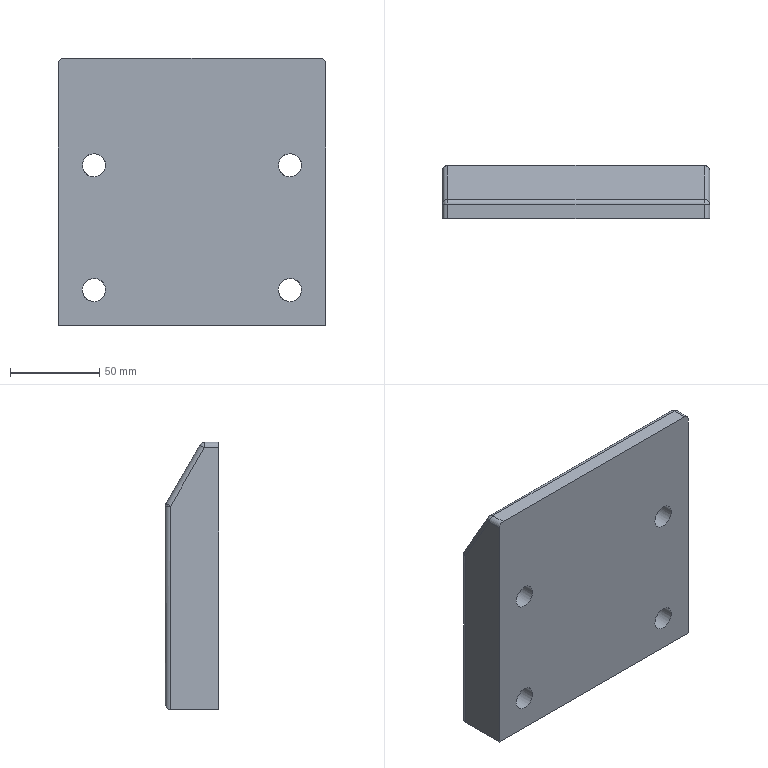Part | NX | features solid 2 | 1 solid | 36 faces | box 150 x 30 x 150 mm | volume 593626 mm3 | cylinder 17 | plane 11 | torus 4 | sphere 4 | commonest cylinder face diameters 6 x9 13 x4 20 x4
STEP:
#1=CARTESIAN_POINT('',(246.5,-620.,-266.5));
#2=VERTEX_POINT('',#1);
#3=CARTESIAN_POINT('',(246.5,-620.,-260.));
#4=DIRECTION('',(0.,1.,0.));
#5=DIRECTION('',(0.,0.,-1.));
#6=AXIS2_PLACEMENT_3D('',#3,#4,#5);
#7=CIRCLE('',#6,6.5);
#8=EDGE_CURVE('',#2,#2,#7,.F.);
#9=ORIENTED_EDGE('',*,*,#8,.F.);
#10=EDGE_LOOP('',(#9));
#11=FACE_BOUND('',#10,.T.);
#12=CARTESIAN_POINT('',(136.5,-620.,-266.5));
#13=VERTEX_POINT('',#12);
#14=CARTESIAN_POINT('',(136.5,-620.,-260.));
#15=DIRECTION('',(0.,1.,0.));
#16=DIRECTION('',(0.,0.,-1.));
#17=AXIS2_PLACEMENT_3D('',#14,#15,#16);
#18=CIRCLE('',#17,6.5);
#19=EDGE_CURVE('',#13,#13,#18,.F.);
#20=ORIENTED_EDGE('',*,*,#19,.F.);
#21=EDGE_LOOP('',(#20));
#22=FACE_BOUND('',#21,.T.);
#23=CARTESIAN_POINT('',(116.5,-620.,-133.));
#24=VERTEX_POINT('',#23);
#25=CARTESIAN_POINT('',(116.5,-620.,-280.));
#26=VERTEX_POINT('',#25);
#27=CARTESIAN_POINT('',(116.5,-620.,-40.));
#28=DIRECTION('',(0.,0.,-1.));
#29=VECTOR('',#28,1000.);
#30=LINE('',#27,#29);
#31=EDGE_CURVE('',#24,#26,#30,.T.);
#32=ORIENTED_EDGE('',*,*,#31,.T.);
#33=CARTESIAN_POINT('',(266.5,-620.,-280.));
#34=VERTEX_POINT('',#33);
#35=CARTESIAN_POINT('',(229.,-620.,-280.));
#36=DIRECTION('',(1.,0.,0.));
#37=VECTOR('',#36,1000.);
#38=LINE('',#35,#37);
#39=EDGE_CURVE('',#26,#34,#38,.T.);
#40=ORIENTED_EDGE('',*,*,#39,.T.);
#41=CARTESIAN_POINT('',(266.5,-620.,-133.));
#42=VERTEX_POINT('',#41);
#43=CARTESIAN_POINT('',(266.5,-620.,-40.));
#44=DIRECTION('',(0.,0.,-1.));
#45=VECTOR('',#44,1000.);
#46=LINE('',#43,#45);
#47=EDGE_CURVE('',#42,#34,#46,.T.);
#48=ORIENTED_EDGE('',*,*,#47,.F.);
#49=CARTESIAN_POINT('',(263.5,-620.,-130.));
#50=VERTEX_POINT('',#49);
#51=CARTESIAN_POINT('',(263.5,-620.,-133.));
#52=DIRECTION('',(0.,1.,0.));
#53=DIRECTION('',(0.,0.,-1.));
#54=AXIS2_PLACEMENT_3D('',#51,#52,#53);
#55=CIRCLE('',#54,3.);
#56=EDGE_CURVE('',#42,#50,#55,.F.);
#57=ORIENTED_EDGE('',*,*,#56,.T.);
#58=CARTESIAN_POINT('',(119.5,-620.,-130.));
#59=VERTEX_POINT('',#58);
#60=CARTESIAN_POINT('',(229.,-620.,-130.));
#61=DIRECTION('',(-1.,0.,0.));
#62=VECTOR('',#61,1000.);
#63=LINE('',#60,#62);
#64=EDGE_CURVE('',#50,#59,#63,.T.);
#65=ORIENTED_EDGE('',*,*,#64,.T.);
#66=CARTESIAN_POINT('',(119.5,-620.,-133.));
#67=DIRECTION('',(0.,1.,0.));
#68=DIRECTION('',(0.,0.,-1.));
#69=AXIS2_PLACEMENT_3D('',#66,#67,#68);
#70=CIRCLE('',#69,3.);
#71=EDGE_CURVE('',#59,#24,#70,.F.);
#72=ORIENTED_EDGE('',*,*,#71,.T.);
#73=EDGE_LOOP('',(#32,#40,#48,#57,#65,#72));
#74=FACE_BOUND('',#73,.T.);
#75=CARTESIAN_POINT('',(246.5,-620.,-196.5));
#76=VERTEX_POINT('',#75);
#77=CARTESIAN_POINT('',(246.5,-620.,-190.));
#78=DIRECTION('',(0.,1.,0.));
#79=DIRECTION('',(0.,0.,-1.));
#80=AXIS2_PLACEMENT_3D('',#77,#78,#79);
#81=CIRCLE('',#80,6.5);
#82=EDGE_CURVE('',#76,#76,#81,.F.);
#83=ORIENTED_EDGE('',*,*,#82,.F.);
#84=EDGE_LOOP('',(#83));
#85=FACE_BOUND('',#84,.T.);
#86=CARTESIAN_POINT('',(136.5,-620.,-196.5));
#87=VERTEX_POINT('',#86);
#88=CARTESIAN_POINT('',(136.5,-620.,-190.));
#89=DIRECTION('',(0.,1.,0.));
#90=DIRECTION('',(0.,0.,-1.));
#91=AXIS2_PLACEMENT_3D('',#88,#89,#90);
#92=CIRCLE('',#91,6.5);
#93=EDGE_CURVE('',#87,#87,#92,.F.);
#94=ORIENTED_EDGE('',*,*,#93,.F.);
#95=EDGE_LOOP('',(#94));
#96=FACE_BOUND('',#95,.T.);
#97=CARTESIAN_POINT('',(-795.,-620.,-162.208));
#98=DIRECTION('',(0.,-1.,0.));
#99=DIRECTION('',(0.,0.,-1.));
#100=AXIS2_PLACEMENT_3D('',#97,#98,#99);
#101=PLANE('',#100);
#102=ADVANCED_FACE('',(#11,#22,#74,#85,#96),#101,.T.);
#103=CARTESIAN_POINT('',(119.5,-590.,-165.804));
#104=VERTEX_POINT('',#103);
#105=CARTESIAN_POINT('',(119.5,-590.,-277.));
#106=VERTEX_POINT('',#105);
#107=CARTESIAN_POINT('',(119.5,-590.,-170.));
#108=DIRECTION('',(0.,0.,1.));
#109=VECTOR('',#108,1000.);
#110=LINE('',#107,#109);
#111=EDGE_CURVE('',#104,#106,#110,.F.);
#112=ORIENTED_EDGE('',*,*,#111,.T.);
#113=CARTESIAN_POINT('',(116.5,-593.,-280.));
#114=VERTEX_POINT('',#113);
#115=CARTESIAN_POINT('',(119.5,-593.,-277.));
#116=DIRECTION('',(0.7071,0.,-0.7071));
#117=DIRECTION('',(-0.7071,0.,-0.7071));
#118=AXIS2_PLACEMENT_3D('',#115,#116,#117);
#119=ELLIPSE('',#118,4.243,3.);
#120=EDGE_CURVE('',#114,#106,#119,.T.);
#121=ORIENTED_EDGE('',*,*,#120,.F.);
#122=CARTESIAN_POINT('',(116.5,-593.,-165.804));
#123=VERTEX_POINT('',#122);
#124=CARTESIAN_POINT('',(116.5,-593.,-40.));
#125=DIRECTION('',(0.,0.,1.));
#126=VECTOR('',#125,1000.);
#127=LINE('',#124,#126);
#128=EDGE_CURVE('',#114,#123,#127,.T.);
#129=ORIENTED_EDGE('',*,*,#128,.T.);
#130=CARTESIAN_POINT('',(119.5,-593.,-165.804));
#131=DIRECTION('',(0.,0.,-1.));
#132=DIRECTION('',(-1.,0.,0.));
#133=AXIS2_PLACEMENT_3D('',#130,#131,#132);
#134=CIRCLE('',#133,3.);
#135=EDGE_CURVE('',#104,#123,#134,.F.);
#136=ORIENTED_EDGE('',*,*,#135,.F.);
#137=EDGE_LOOP('',(#112,#121,#129,#136));
#138=FACE_BOUND('',#137,.T.);
#139=CARTESIAN_POINT('',(119.5,-593.,-40.));
#140=DIRECTION('',(0.,0.,1.));
#141=DIRECTION('',(-1.,0.,0.));
#142=AXIS2_PLACEMENT_3D('',#139,#140,#141);
#143=CYLINDRICAL_SURFACE('',#142,3.);
#144=ADVANCED_FACE('',(#138),#143,.T.);
#145=CARTESIAN_POINT('',(266.5,-593.,-165.804));
#146=VERTEX_POINT('',#145);
#147=CARTESIAN_POINT('',(266.5,-593.,-280.));
#148=VERTEX_POINT('',#147);
#149=CARTESIAN_POINT('',(266.5,-593.,-170.));
#150=DIRECTION('',(0.,0.,1.));
#151=VECTOR('',#150,1000.);
#152=LINE('',#149,#151);
#153=EDGE_CURVE('',#146,#148,#152,.F.);
#154=ORIENTED_EDGE('',*,*,#153,.T.);
#155=CARTESIAN_POINT('',(263.5,-590.,-277.));
#156=VERTEX_POINT('',#155);
#157=CARTESIAN_POINT('',(263.5,-593.,-277.));
#158=DIRECTION('',(0.7071,0.,0.7071));
#159=DIRECTION('',(-0.7071,0.,0.7071));
#160=AXIS2_PLACEMENT_3D('',#157,#158,#159);
#161=ELLIPSE('',#160,4.243,3.);
#162=EDGE_CURVE('',#148,#156,#161,.T.);
#163=ORIENTED_EDGE('',*,*,#162,.T.);
#164=CARTESIAN_POINT('',(263.5,-590.,-165.804));
#165=VERTEX_POINT('',#164);
#166=CARTESIAN_POINT('',(263.5,-590.,-75.));
#167=DIRECTION('',(0.,0.,1.));
#168=VECTOR('',#167,1000.);
#169=LINE('',#166,#168);
#170=EDGE_CURVE('',#156,#165,#169,.T.);
#171=ORIENTED_EDGE('',*,*,#170,.T.);
#172=CARTESIAN_POINT('',(263.5,-593.,-165.804));
#173=DIRECTION('',(0.,0.,-1.));
#174=DIRECTION('',(-1.,0.,0.));
#175=AXIS2_PLACEMENT_3D('',#172,#173,#174);
#176=CIRCLE('',#175,3.);
#177=EDGE_CURVE('',#146,#165,#176,.F.);
#178=ORIENTED_EDGE('',*,*,#177,.F.);
#179=EDGE_LOOP('',(#154,#163,#171,#178));
#180=FACE_BOUND('',#179,.T.);
#181=CARTESIAN_POINT('',(263.5,-593.,-170.));
#182=DIRECTION('',(0.,0.,-1.));
#183=DIRECTION('',(1.,0.,0.));
#184=AXIS2_PLACEMENT_3D('',#181,#182,#183);
#185=CYLINDRICAL_SURFACE('',#184,3.);
#186=ADVANCED_FACE('',(#180),#185,.T.);
#187=CARTESIAN_POINT('',(259.5,-590.,-260.));
#188=VERTEX_POINT('',#187);
#189=CARTESIAN_POINT('',(246.5,-590.,-260.));
#190=DIRECTION('',(0.,-1.,0.));
#191=DIRECTION('',(1.,0.,0.));
#192=AXIS2_PLACEMENT_3D('',#189,#190,#191);
#193=CIRCLE('',#192,13.);
#194=EDGE_CURVE('',#188,#188,#193,.F.);
#195=ORIENTED_EDGE('',*,*,#194,.F.);
#196=EDGE_LOOP('',(#195));
#197=FACE_BOUND('',#196,.T.);
#198=CARTESIAN_POINT('',(149.5,-590.,-260.));
#199=VERTEX_POINT('',#198);
#200=CARTESIAN_POINT('',(136.5,-590.,-260.));
#201=DIRECTION('',(0.,-1.,0.));
#202=DIRECTION('',(1.,0.,0.));
#203=AXIS2_PLACEMENT_3D('',#200,#201,#202);
#204=CIRCLE('',#203,13.);
#205=EDGE_CURVE('',#199,#199,#204,.F.);
#206=ORIENTED_EDGE('',*,*,#205,.F.);
#207=EDGE_LOOP('',(#206));
#208=FACE_BOUND('',#207,.T.);
#209=ORIENTED_EDGE('',*,*,#170,.F.);
#210=CARTESIAN_POINT('',(229.,-590.,-277.));
#211=DIRECTION('',(-1.,0.,0.));
#212=VECTOR('',#211,1000.);
#213=LINE('',#210,#212);
#214=EDGE_CURVE('',#106,#156,#213,.F.);
#215=ORIENTED_EDGE('',*,*,#214,.F.);
#216=ORIENTED_EDGE('',*,*,#111,.F.);
#217=CARTESIAN_POINT('',(229.,-590.,-165.804));
#218=DIRECTION('',(-1.,0.,0.));
#219=VECTOR('',#218,1000.);
#220=LINE('',#217,#219);
#221=EDGE_CURVE('',#165,#104,#220,.T.);
#222=ORIENTED_EDGE('',*,*,#221,.F.);
#223=EDGE_LOOP('',(#209,#215,#216,#222));
#224=FACE_BOUND('',#223,.T.);
#225=CARTESIAN_POINT('',(259.5,-590.,-190.));
#226=VERTEX_POINT('',#225);
#227=CARTESIAN_POINT('',(246.5,-590.,-190.));
#228=DIRECTION('',(0.,-1.,0.));
#229=DIRECTION('',(1.,0.,0.));
#230=AXIS2_PLACEMENT_3D('',#227,#228,#229);
#231=CIRCLE('',#230,13.);
#232=EDGE_CURVE('',#226,#226,#231,.F.);
#233=ORIENTED_EDGE('',*,*,#232,.F.);
#234=EDGE_LOOP('',(#233));
#235=FACE_BOUND('',#234,.T.);
#236=CARTESIAN_POINT('',(149.5,-590.,-190.));
#237=VERTEX_POINT('',#236);
#238=CARTESIAN_POINT('',(136.5,-590.,-190.));
#239=DIRECTION('',(0.,-1.,0.));
#240=DIRECTION('',(1.,0.,0.));
#241=AXIS2_PLACEMENT_3D('',#238,#239,#240);
#242=CIRCLE('',#241,13.);
#243=EDGE_CURVE('',#237,#237,#242,.F.);
#244=ORIENTED_EDGE('',*,*,#243,.F.);
#245=EDGE_LOOP('',(#244));
#246=FACE_BOUND('',#245,.T.);
#247=CARTESIAN_POINT('',(229.,-590.,-170.));
#248=DIRECTION('',(0.,1.,0.));
#249=DIRECTION('',(1.,0.,0.));
#250=AXIS2_PLACEMENT_3D('',#247,#248,#249);
#251=PLANE('',#250);
#252=ADVANCED_FACE('',(#197,#208,#224,#235,#246),#251,.T.);
#253=ORIENTED_EDGE('',*,*,#128,.F.);
#254=CARTESIAN_POINT('',(116.5,-620.,-280.));
#255=DIRECTION('',(0.,1.,0.));
#256=VECTOR('',#255,1000.);
#257=LINE('',#254,#256);
#258=EDGE_CURVE('',#26,#114,#257,.T.);
#259=ORIENTED_EDGE('',*,*,#258,.F.);
#260=ORIENTED_EDGE('',*,*,#31,.F.);
#261=CARTESIAN_POINT('',(116.5,-611.939,-133.));
#262=VERTEX_POINT('',#261);
#263=CARTESIAN_POINT('',(116.5,-590.,-133.));
#264=DIRECTION('',(0.,-1.,0.));
#265=VECTOR('',#264,1000.);
#266=LINE('',#263,#265);
#267=EDGE_CURVE('',#262,#24,#266,.T.);
#268=ORIENTED_EDGE('',*,*,#267,.F.);
#269=CARTESIAN_POINT('',(116.5,-607.754,-140.25));
#270=DIRECTION('',(0.,-0.5,0.866));
#271=VECTOR('',#270,1000.);
#272=LINE('',#269,#271);
#273=EDGE_CURVE('',#123,#262,#272,.T.);
#274=ORIENTED_EDGE('',*,*,#273,.F.);
#275=EDGE_LOOP('',(#253,#259,#260,#268,#274));
#276=FACE_BOUND('',#275,.T.);
#277=CARTESIAN_POINT('',(116.5,-590.,-40.));
#278=DIRECTION('',(-1.,0.,0.));
#279=DIRECTION('',(0.,0.,-1.));
#280=AXIS2_PLACEMENT_3D('',#277,#278,#279);
#281=PLANE('',#280);
#282=ADVANCED_FACE('',(#276),#281,.T.);
#283=ORIENTED_EDGE('',*,*,#47,.T.);
#284=CARTESIAN_POINT('',(266.5,-620.,-280.));
#285=DIRECTION('',(0.,1.,0.));
#286=VECTOR('',#285,1000.);
#287=LINE('',#284,#286);
#288=EDGE_CURVE('',#34,#148,#287,.T.);
#289=ORIENTED_EDGE('',*,*,#288,.T.);
#290=ORIENTED_EDGE('',*,*,#153,.F.);
#291=CARTESIAN_POINT('',(266.5,-611.939,-133.));
#292=VERTEX_POINT('',#291);
#293=CARTESIAN_POINT('',(266.5,-592.598,-166.5));
#294=DIRECTION('',(0.,-0.5,0.866));
#295=VECTOR('',#294,1000.);
#296=LINE('',#293,#295);
#297=EDGE_CURVE('',#292,#146,#296,.F.);
#298=ORIENTED_EDGE('',*,*,#297,.F.);
#299=CARTESIAN_POINT('',(266.5,-610.207,-133.));
#300=DIRECTION('',(0.,-1.,0.));
#301=VECTOR('',#300,1000.);
#302=LINE('',#299,#301);
#303=EDGE_CURVE('',#42,#292,#302,.F.);
#304=ORIENTED_EDGE('',*,*,#303,.F.);
#305=EDGE_LOOP('',(#283,#289,#290,#298,#304));
#306=FACE_BOUND('',#305,.T.);
#307=CARTESIAN_POINT('',(266.5,-590.,-40.));
#308=DIRECTION('',(-1.,0.,0.));
#309=DIRECTION('',(0.,0.,-1.));
#310=AXIS2_PLACEMENT_3D('',#307,#308,#309);
#311=PLANE('',#310);
#312=ADVANCED_FACE('',(#306),#311,.F.);
#313=CARTESIAN_POINT('',(256.5,-593.,-260.));
#314=VERTEX_POINT('',#313);
#315=CARTESIAN_POINT('',(246.5,-593.,-260.));
#316=DIRECTION('',(0.,-1.,0.));
#317=DIRECTION('',(1.,0.,0.));
#318=AXIS2_PLACEMENT_3D('',#315,#316,#317);
#319=CIRCLE('',#318,10.);
#320=EDGE_CURVE('',#314,#314,#319,.T.);
#321=ORIENTED_EDGE('',*,*,#320,.F.);
#322=EDGE_LOOP('',(#321));
#323=FACE_BOUND('',#322,.T.);
#324=CARTESIAN_POINT('',(236.5,-605.,-260.));
#325=VERTEX_POINT('',#324);
#326=CARTESIAN_POINT('',(246.5,-605.,-260.));
#327=DIRECTION('',(0.,1.,0.));
#328=DIRECTION('',(-1.,0.,0.));
#329=AXIS2_PLACEMENT_3D('',#326,#327,#328);
#330=CIRCLE('',#329,10.);
#331=EDGE_CURVE('',#325,#325,#330,.T.);
#332=ORIENTED_EDGE('',*,*,#331,.F.);
#333=EDGE_LOOP('',(#332));
#334=FACE_BOUND('',#333,.T.);
#335=CARTESIAN_POINT('',(246.5,-590.,-260.));
#336=DIRECTION('',(0.,-1.,0.));
#337=DIRECTION('',(-1.,0.,0.));
#338=AXIS2_PLACEMENT_3D('',#335,#336,#337);
#339=CYLINDRICAL_SURFACE('',#338,10.);
#340=ADVANCED_FACE('',(#323,#334),#339,.F.);
#341=CARTESIAN_POINT('',(146.5,-593.,-260.));
#342=VERTEX_POINT('',#341);
#343=CARTESIAN_POINT('',(136.5,-593.,-260.));
#344=DIRECTION('',(0.,-1.,0.));
#345=DIRECTION('',(1.,0.,0.));
#346=AXIS2_PLACEMENT_3D('',#343,#344,#345);
#347=CIRCLE('',#346,10.);
#348=EDGE_CURVE('',#342,#342,#347,.T.);
#349=ORIENTED_EDGE('',*,*,#348,.F.);
#350=EDGE_LOOP('',(#349));
#351=FACE_BOUND('',#350,.T.);
#352=CARTESIAN_POINT('',(126.5,-605.,-260.));
#353=VERTEX_POINT('',#352);
#354=CARTESIAN_POINT('',(136.5,-605.,-260.));
#355=DIRECTION('',(0.,1.,0.));
#356=DIRECTION('',(-1.,0.,0.));
#357=AXIS2_PLACEMENT_3D('',#354,#355,#356);
#358=CIRCLE('',#357,10.);
#359=EDGE_CURVE('',#353,#353,#358,.T.);
#360=ORIENTED_EDGE('',*,*,#359,.F.);
#361=EDGE_LOOP('',(#360));
#362=FACE_BOUND('',#361,.T.);
#363=CARTESIAN_POINT('',(136.5,-590.,-260.));
#364=DIRECTION('',(0.,-1.,0.));
#365=DIRECTION('',(-1.,0.,0.));
#366=AXIS2_PLACEMENT_3D('',#363,#364,#365);
#367=CYLINDRICAL_SURFACE('',#366,10.);
#368=ADVANCED_FACE('',(#351,#362),#367,.F.);
#369=CARTESIAN_POINT('',(240.,-605.,-260.));
#370=VERTEX_POINT('',#369);
#371=CARTESIAN_POINT('',(246.5,-605.,-260.));
#372=DIRECTION('',(0.,1.,0.));
#373=DIRECTION('',(-1.,0.,0.));
#374=AXIS2_PLACEMENT_3D('',#371,#372,#373);
#375=CIRCLE('',#374,6.5);
#376=EDGE_CURVE('',#370,#370,#375,.T.);
#377=ORIENTED_EDGE('',*,*,#376,.F.);
#378=EDGE_LOOP('',(#377));
#379=FACE_BOUND('',#378,.T.);
#380=ORIENTED_EDGE('',*,*,#331,.T.);
#381=EDGE_LOOP('',(#380));
#382=FACE_BOUND('',#381,.T.);
#383=CARTESIAN_POINT('',(211.5,-605.,-150.));
#384=DIRECTION('',(0.,-1.,0.));
#385=DIRECTION('',(-1.,0.,0.));
#386=AXIS2_PLACEMENT_3D('',#383,#384,#385);
#387=PLANE('',#386);
#388=ADVANCED_FACE('',(#379,#382),#387,.F.);
#389=CARTESIAN_POINT('',(130.,-605.,-260.));
#390=VERTEX_POINT('',#389);
#391=CARTESIAN_POINT('',(136.5,-605.,-260.));
#392=DIRECTION('',(0.,1.,0.));
#393=DIRECTION('',(-1.,0.,0.));
#394=AXIS2_PLACEMENT_3D('',#391,#392,#393);
#395=CIRCLE('',#394,6.5);
#396=EDGE_CURVE('',#390,#390,#395,.T.);
#397=ORIENTED_EDGE('',*,*,#396,.F.);
#398=EDGE_LOOP('',(#397));
#399=FACE_BOUND('',#398,.T.);
#400=ORIENTED_EDGE('',*,*,#359,.T.);
#401=EDGE_LOOP('',(#400));
#402=FACE_BOUND('',#401,.T.);
#403=CARTESIAN_POINT('',(171.5,-605.,-150.));
#404=DIRECTION('',(0.,-1.,0.));
#405=DIRECTION('',(-1.,0.,0.));
#406=AXIS2_PLACEMENT_3D('',#403,#404,#405);
#407=PLANE('',#406);
#408=ADVANCED_FACE('',(#399,#402),#407,.F.);
#409=ORIENTED_EDGE('',*,*,#320,.T.);
#410=EDGE_LOOP('',(#409));
#411=FACE_BOUND('',#410,.T.);
#412=ORIENTED_EDGE('',*,*,#194,.T.);
#413=EDGE_LOOP('',(#412));
#414=FACE_BOUND('',#413,.T.);
#415=CARTESIAN_POINT('',(246.5,-593.,-260.));
#416=DIRECTION('',(0.,1.,0.));
#417=DIRECTION('',(1.,0.,0.));
#418=AXIS2_PLACEMENT_3D('',#415,#416,#417);
#419=TOROIDAL_SURFACE('',#418,13.,3.);
#420=ADVANCED_FACE('',(#411,#414),#419,.T.);
#421=ORIENTED_EDGE('',*,*,#348,.T.);
#422=EDGE_LOOP('',(#421));
#423=FACE_BOUND('',#422,.T.);
#424=ORIENTED_EDGE('',*,*,#205,.T.);
#425=EDGE_LOOP('',(#424));
#426=FACE_BOUND('',#425,.T.);
#427=CARTESIAN_POINT('',(136.5,-593.,-260.));
#428=DIRECTION('',(0.,1.,0.));
#429=DIRECTION('',(1.,0.,0.));
#430=AXIS2_PLACEMENT_3D('',#427,#428,#429);
#431=TOROIDAL_SURFACE('',#430,13.,3.);
#432=ADVANCED_FACE('',(#423,#426),#431,.T.);
#433=ORIENTED_EDGE('',*,*,#162,.F.);
#434=CARTESIAN_POINT('',(229.,-593.,-280.));
#435=DIRECTION('',(-1.,0.,0.));
#436=VECTOR('',#435,1000.);
#437=LINE('',#434,#436);
#438=EDGE_CURVE('',#148,#114,#437,.T.);
#439=ORIENTED_EDGE('',*,*,#438,.T.);
#440=ORIENTED_EDGE('',*,*,#120,.T.);
#441=ORIENTED_EDGE('',*,*,#214,.T.);
#442=EDGE_LOOP('',(#433,#439,#440,#441));
#443=FACE_BOUND('',#442,.T.);
#444=CARTESIAN_POINT('',(229.,-593.,-277.));
#445=DIRECTION('',(-1.,0.,0.));
#446=DIRECTION('',(0.,0.,-1.));
#447=AXIS2_PLACEMENT_3D('',#444,#445,#446);
#448=CYLINDRICAL_SURFACE('',#447,3.);
#449=ADVANCED_FACE('',(#443),#448,.T.);
#450=ORIENTED_EDGE('',*,*,#258,.T.);
#451=ORIENTED_EDGE('',*,*,#438,.F.);
#452=ORIENTED_EDGE('',*,*,#288,.F.);
#453=ORIENTED_EDGE('',*,*,#39,.F.);
#454=EDGE_LOOP('',(#450,#451,#452,#453));
#455=FACE_BOUND('',#454,.T.);
#456=CARTESIAN_POINT('',(229.,-620.,-280.));
#457=DIRECTION('',(0.,0.,-1.));
#458=DIRECTION('',(1.,0.,0.));
#459=AXIS2_PLACEMENT_3D('',#456,#457,#458);
#460=PLANE('',#459);
#461=ADVANCED_FACE('',(#455),#460,.T.);
#462=ORIENTED_EDGE('',*,*,#376,.T.);
#463=EDGE_LOOP('',(#462));
#464=FACE_BOUND('',#463,.T.);
#465=ORIENTED_EDGE('',*,*,#8,.T.);
#466=EDGE_LOOP('',(#465));
#467=FACE_BOUND('',#466,.T.);
#468=CARTESIAN_POINT('',(246.5,-620.,-260.));
#469=DIRECTION('',(0.,-1.,0.));
#470=DIRECTION('',(-1.,0.,0.));
#471=AXIS2_PLACEMENT_3D('',#468,#469,#470);
#472=CYLINDRICAL_SURFACE('',#471,6.5);
#473=ADVANCED_FACE('',(#464,#467),#472,.F.);
#474=ORIENTED_EDGE('',*,*,#396,.T.);
#475=EDGE_LOOP('',(#474));
#476=FACE_BOUND('',#475,.T.);
#477=ORIENTED_EDGE('',*,*,#19,.T.);
#478=EDGE_LOOP('',(#477));
#479=FACE_BOUND('',#478,.T.);
#480=CARTESIAN_POINT('',(136.5,-620.,-260.));
#481=DIRECTION('',(0.,-1.,0.));
#482=DIRECTION('',(-1.,0.,0.));
#483=AXIS2_PLACEMENT_3D('',#480,#481,#482);
#484=CYLINDRICAL_SURFACE('',#483,6.5);
#485=ADVANCED_FACE('',(#476,#479),#484,.F.);
#486=CARTESIAN_POINT('',(263.5,-611.939,-130.));
#487=VERTEX_POINT('',#486);
#488=CARTESIAN_POINT('',(263.5,-620.,-130.));
#489=DIRECTION('',(0.,-1.,0.));
#490=VECTOR('',#489,1000.);
#491=LINE('',#488,#490);
#492=EDGE_CURVE('',#487,#50,#491,.T.);
#493=ORIENTED_EDGE('',*,*,#492,.F.);
#494=CARTESIAN_POINT('',(119.5,-611.939,-130.));
#495=VERTEX_POINT('',#494);
#496=CARTESIAN_POINT('',(229.,-611.939,-130.));
#497=DIRECTION('',(-1.,0.,0.));
#498=VECTOR('',#497,1000.);
#499=LINE('',#496,#498);
#500=EDGE_CURVE('',#495,#487,#499,.F.);
#501=ORIENTED_EDGE('',*,*,#500,.F.);
#502=CARTESIAN_POINT('',(119.5,-610.207,-130.));
#503=DIRECTION('',(0.,-1.,0.));
#504=VECTOR('',#503,1000.);
#505=LINE('',#502,#504);
#506=EDGE_CURVE('',#59,#495,#505,.F.);
#507=ORIENTED_EDGE('',*,*,#506,.F.);
#508=ORIENTED_EDGE('',*,*,#64,.F.);
#509=EDGE_LOOP('',(#493,#501,#507,#508));
#510=FACE_BOUND('',#509,.T.);
#511=CARTESIAN_POINT('',(229.,-610.207,-130.));
#512=DIRECTION('',(0.,0.,1.));
#513=DIRECTION('',(-1.,0.,0.));
#514=AXIS2_PLACEMENT_3D('',#511,#512,#513);
#515=PLANE('',#514);
#516=ADVANCED_FACE('',(#510),#515,.T.);
#517=CARTESIAN_POINT('',(130.,-605.,-190.));
#518=VERTEX_POINT('',#517);
#519=CARTESIAN_POINT('',(136.5,-605.,-190.));
#520=DIRECTION('',(0.,1.,0.));
#521=DIRECTION('',(-1.,0.,0.));
#522=AXIS2_PLACEMENT_3D('',#519,#520,#521);
#523=CIRCLE('',#522,6.5);
#524=EDGE_CURVE('',#518,#518,#523,.T.);
#525=ORIENTED_EDGE('',*,*,#524,.T.);
#526=EDGE_LOOP('',(#525));
#527=FACE_BOUND('',#526,.T.);
#528=ORIENTED_EDGE('',*,*,#93,.T.);
#529=EDGE_LOOP('',(#528));
#530=FACE_BOUND('',#529,.T.);
#531=CARTESIAN_POINT('',(136.5,-620.,-190.));
#532=DIRECTION('',(0.,-1.,0.));
#533=DIRECTION('',(-1.,0.,0.));
#534=AXIS2_PLACEMENT_3D('',#531,#532,#533);
#535=CYLINDRICAL_SURFACE('',#534,6.5);
#536=ADVANCED_FACE('',(#527,#530),#535,.F.);
#537=CARTESIAN_POINT('',(240.,-605.,-190.));
#538=VERTEX_POINT('',#537);
#539=CARTESIAN_POINT('',(246.5,-605.,-190.));
#540=DIRECTION('',(0.,1.,0.));
#541=DIRECTION('',(-1.,0.,0.));
#542=AXIS2_PLACEMENT_3D('',#539,#540,#541);
#543=CIRCLE('',#542,6.5);
#544=EDGE_CURVE('',#538,#538,#543,.T.);
#545=ORIENTED_EDGE('',*,*,#544,.T.);
#546=EDGE_LOOP('',(#545));
#547=FACE_BOUND('',#546,.T.);
#548=ORIENTED_EDGE('',*,*,#82,.T.);
#549=EDGE_LOOP('',(#548));
#550=FACE_BOUND('',#549,.T.);
#551=CARTESIAN_POINT('',(246.5,-620.,-190.));
#552=DIRECTION('',(0.,-1.,0.));
#553=DIRECTION('',(-1.,0.,0.));
#554=AXIS2_PLACEMENT_3D('',#551,#552,#553);
#555=CYLINDRICAL_SURFACE('',#554,6.5);
#556=ADVANCED_FACE('',(#547,#550),#555,.F.);
#557=ORIENTED_EDGE('',*,*,#303,.T.);
#558=CARTESIAN_POINT('',(263.5,-611.939,-133.));
#559=DIRECTION('',(0.,-1.,0.));
#560=DIRECTION('',(0.,0.,-1.));
#561=AXIS2_PLACEMENT_3D('',#558,#559,#560);
#562=CIRCLE('',#561,3.);
#563=EDGE_CURVE('',#292,#487,#562,.T.);
#564=ORIENTED_EDGE('',*,*,#563,.T.);
#565=ORIENTED_EDGE('',*,*,#492,.T.);
#566=ORIENTED_EDGE('',*,*,#56,.F.);
#567=EDGE_LOOP('',(#557,#564,#565,#566));
#568=FACE_BOUND('',#567,.T.);
#569=CARTESIAN_POINT('',(263.5,-610.207,-133.));
#570=DIRECTION('',(0.,1.,0.));
#571=DIRECTION('',(1.,0.,0.));
#572=AXIS2_PLACEMENT_3D('',#569,#570,#571);
#573=CYLINDRICAL_SURFACE('',#572,3.);
#574=ADVANCED_FACE('',(#568),#573,.T.);
#575=ORIENTED_EDGE('',*,*,#506,.T.);
#576=CARTESIAN_POINT('',(119.5,-611.939,-133.));
#577=DIRECTION('',(0.,-1.,0.));
#578=DIRECTION('',(1.,0.,0.));
#579=AXIS2_PLACEMENT_3D('',#576,#577,#578);
#580=CIRCLE('',#579,3.);
#581=EDGE_CURVE('',#495,#262,#580,.T.);
#582=ORIENTED_EDGE('',*,*,#581,.T.);
#583=ORIENTED_EDGE('',*,*,#267,.T.);
#584=ORIENTED_EDGE('',*,*,#71,.F.);
#585=EDGE_LOOP('',(#575,#582,#583,#584));
#586=FACE_BOUND('',#585,.T.);
#587=CARTESIAN_POINT('',(119.5,-590.,-133.));
#588=DIRECTION('',(0.,-1.,0.));
#589=DIRECTION('',(-1.,0.,0.));
#590=AXIS2_PLACEMENT_3D('',#587,#588,#589);
#591=CYLINDRICAL_SURFACE('',#590,3.);
#592=ADVANCED_FACE('',(#586),#591,.T.);
#593=CARTESIAN_POINT('',(263.5,-590.402,-164.304));
#594=VERTEX_POINT('',#593);
#595=CARTESIAN_POINT('',(263.5,-609.341,-131.5));
#596=VERTEX_POINT('',#595);
#597=CARTESIAN_POINT('',(263.5,-610.207,-130.));
#598=DIRECTION('',(0.,-0.5,0.866));
#599=VECTOR('',#598,1000.);
#600=LINE('',#597,#599);
#601=EDGE_CURVE('',#594,#596,#600,.T.);
#602=ORIENTED_EDGE('',*,*,#601,.F.);
#603=CARTESIAN_POINT('',(119.5,-590.402,-164.304));
#604=VERTEX_POINT('',#603);
#605=CARTESIAN_POINT('',(229.,-590.402,-164.304));
#606=DIRECTION('',(-1.,0.,0.));
#607=VECTOR('',#606,1000.);
#608=LINE('',#605,#607);
#609=EDGE_CURVE('',#604,#594,#608,.F.);
#610=ORIENTED_EDGE('',*,*,#609,.F.);
#611=CARTESIAN_POINT('',(119.5,-609.341,-131.5));
#612=VERTEX_POINT('',#611);
#613=CARTESIAN_POINT('',(119.5,-590.,-165.));
#614=DIRECTION('',(0.,-0.5,0.866));
#615=VECTOR('',#614,1000.);
#616=LINE('',#613,#615);
#617=EDGE_CURVE('',#612,#604,#616,.F.);
#618=ORIENTED_EDGE('',*,*,#617,.F.);
#619=CARTESIAN_POINT('',(229.,-609.341,-131.5));
#620=DIRECTION('',(-1.,0.,0.));
#621=VECTOR('',#620,1000.);
#622=LINE('',#619,#621);
#623=EDGE_CURVE('',#596,#612,#622,.T.);
#624=ORIENTED_EDGE('',*,*,#623,.F.);
#625=EDGE_LOOP('',(#602,#610,#618,#624));
#626=FACE_BOUND('',#625,.T.);
#627=CARTESIAN_POINT('',(229.,-590.,-165.));
#628=DIRECTION('',(0.,0.866,0.5));
#629=DIRECTION('',(0.,0.5,-0.866));
#630=AXIS2_PLACEMENT_3D('',#627,#628,#629);
#631=PLANE('',#630);
#632=ADVANCED_FACE('',(#626),#631,.T.);
#633=ORIENTED_EDGE('',*,*,#524,.F.);
#634=EDGE_LOOP('',(#633));
#635=FACE_BOUND('',#634,.T.);
#636=CARTESIAN_POINT('',(126.5,-605.,-190.));
#637=VERTEX_POINT('',#636);
#638=CARTESIAN_POINT('',(136.5,-605.,-190.));
#639=DIRECTION('',(0.,1.,0.));
#640=DIRECTION('',(-1.,0.,0.));
#641=AXIS2_PLACEMENT_3D('',#638,#639,#640);
#642=CIRCLE('',#641,10.);
#643=EDGE_CURVE('',#637,#637,#642,.T.);
#644=ORIENTED_EDGE('',*,*,#643,.T.);
#645=EDGE_LOOP('',(#644));
#646=FACE_BOUND('',#645,.T.);
#647=CARTESIAN_POINT('',(171.5,-605.,-190.));
#648=DIRECTION('',(0.,-1.,0.));
#649=DIRECTION('',(-1.,0.,0.));
#650=AXIS2_PLACEMENT_3D('',#647,#648,#649);
#651=PLANE('',#650);
#652=ADVANCED_FACE('',(#635,#646),#651,.F.);
#653=CARTESIAN_POINT('',(146.5,-593.,-190.));
#654=VERTEX_POINT('',#653);
#655=CARTESIAN_POINT('',(136.5,-593.,-190.));
#656=DIRECTION('',(0.,-1.,0.));
#657=DIRECTION('',(1.,0.,0.));
#658=AXIS2_PLACEMENT_3D('',#655,#656,#657);
#659=CIRCLE('',#658,10.);
#660=EDGE_CURVE('',#654,#654,#659,.T.);
#661=ORIENTED_EDGE('',*,*,#660,.F.);
#662=EDGE_LOOP('',(#661));
#663=FACE_BOUND('',#662,.T.);
#664=ORIENTED_EDGE('',*,*,#643,.F.);
#665=EDGE_LOOP('',(#664));
#666=FACE_BOUND('',#665,.T.);
#667=CARTESIAN_POINT('',(136.5,-590.,-190.));
#668=DIRECTION('',(0.,-1.,0.));
#669=DIRECTION('',(-1.,0.,0.));
#670=AXIS2_PLACEMENT_3D('',#667,#668,#669);
#671=CYLINDRICAL_SURFACE('',#670,10.);
#672=ADVANCED_FACE('',(#663,#666),#671,.F.);
#673=ORIENTED_EDGE('',*,*,#544,.F.);
#674=EDGE_LOOP('',(#673));
#675=FACE_BOUND('',#674,.T.);
#676=CARTESIAN_POINT('',(236.5,-605.,-190.));
#677=VERTEX_POINT('',#676);
#678=CARTESIAN_POINT('',(246.5,-605.,-190.));
#679=DIRECTION('',(0.,1.,0.));
#680=DIRECTION('',(-1.,0.,0.));
#681=AXIS2_PLACEMENT_3D('',#678,#679,#680);
#682=CIRCLE('',#681,10.);
#683=EDGE_CURVE('',#677,#677,#682,.T.);
#684=ORIENTED_EDGE('',*,*,#683,.T.);
#685=EDGE_LOOP('',(#684));
#686=FACE_BOUND('',#685,.T.);
#687=CARTESIAN_POINT('',(211.5,-605.,-190.));
#688=DIRECTION('',(0.,-1.,0.));
#689=DIRECTION('',(-1.,0.,0.));
#690=AXIS2_PLACEMENT_3D('',#687,#688,#689);
#691=PLANE('',#690);
#692=ADVANCED_FACE('',(#675,#686),#691,.F.);
#693=CARTESIAN_POINT('',(256.5,-593.,-190.));
#694=VERTEX_POINT('',#693);
#695=CARTESIAN_POINT('',(246.5,-593.,-190.));
#696=DIRECTION('',(0.,-1.,0.));
#697=DIRECTION('',(1.,0.,0.));
#698=AXIS2_PLACEMENT_3D('',#695,#696,#697);
#699=CIRCLE('',#698,10.);
#700=EDGE_CURVE('',#694,#694,#699,.T.);
#701=ORIENTED_EDGE('',*,*,#700,.F.);
#702=EDGE_LOOP('',(#701));
#703=FACE_BOUND('',#702,.T.);
#704=ORIENTED_EDGE('',*,*,#683,.F.);
#705=EDGE_LOOP('',(#704));
#706=FACE_BOUND('',#705,.T.);
#707=CARTESIAN_POINT('',(246.5,-590.,-190.));
#708=DIRECTION('',(0.,-1.,0.));
#709=DIRECTION('',(-1.,0.,0.));
#710=AXIS2_PLACEMENT_3D('',#707,#708,#709);
#711=CYLINDRICAL_SURFACE('',#710,10.);
#712=ADVANCED_FACE('',(#703,#706),#711,.F.);
#713=ORIENTED_EDGE('',*,*,#700,.T.);
#714=EDGE_LOOP('',(#713));
#715=FACE_BOUND('',#714,.T.);
#716=ORIENTED_EDGE('',*,*,#232,.T.);
#717=EDGE_LOOP('',(#716));
#718=FACE_BOUND('',#717,.T.);
#719=CARTESIAN_POINT('',(246.5,-593.,-190.));
#720=DIRECTION('',(0.,1.,0.));
#721=DIRECTION('',(1.,0.,0.));
#722=AXIS2_PLACEMENT_3D('',#719,#720,#721);
#723=TOROIDAL_SURFACE('',#722,13.,3.);
#724=ADVANCED_FACE('',(#715,#718),#723,.T.);
#725=ORIENTED_EDGE('',*,*,#660,.T.);
#726=EDGE_LOOP('',(#725));
#727=FACE_BOUND('',#726,.T.);
#728=ORIENTED_EDGE('',*,*,#243,.T.);
#729=EDGE_LOOP('',(#728));
#730=FACE_BOUND('',#729,.T.);
#731=CARTESIAN_POINT('',(136.5,-593.,-190.));
#732=DIRECTION('',(0.,1.,0.));
#733=DIRECTION('',(1.,0.,0.));
#734=AXIS2_PLACEMENT_3D('',#731,#732,#733);
#735=TOROIDAL_SURFACE('',#734,13.,3.);
#736=ADVANCED_FACE('',(#727,#730),#735,.T.);
#737=CARTESIAN_POINT('',(263.5,-611.939,-133.));
#738=DIRECTION('',(0.,0.5,-0.866));
#739=DIRECTION('',(0.,0.866,0.5));
#740=AXIS2_PLACEMENT_3D('',#737,#738,#739);
#741=CIRCLE('',#740,3.);
#742=EDGE_CURVE('',#292,#596,#741,.F.);
#743=ORIENTED_EDGE('',*,*,#742,.T.);
#744=CARTESIAN_POINT('',(263.5,-611.939,-133.));
#745=DIRECTION('',(-1.,0.,0.));
#746=DIRECTION('',(0.,0.,1.));
#747=AXIS2_PLACEMENT_3D('',#744,#745,#746);
#748=CIRCLE('',#747,3.);
#749=EDGE_CURVE('',#596,#487,#748,.F.);
#750=ORIENTED_EDGE('',*,*,#749,.T.);
#751=ORIENTED_EDGE('',*,*,#563,.F.);
#752=EDGE_LOOP('',(#743,#750,#751));
#753=FACE_BOUND('',#752,.T.);
#754=CARTESIAN_POINT('',(263.5,-611.939,-133.));
#755=DIRECTION('',(1.,0.,0.));
#756=DIRECTION('',(0.,0.,1.));
#757=AXIS2_PLACEMENT_3D('',#754,#755,#756);
#758=SPHERICAL_SURFACE('',#757,3.);
#759=ADVANCED_FACE('',(#753),#758,.T.);
#760=ORIENTED_EDGE('',*,*,#749,.F.);
#761=ORIENTED_EDGE('',*,*,#623,.T.);
#762=CARTESIAN_POINT('',(119.5,-611.939,-133.));
#763=DIRECTION('',(1.,0.,0.));
#764=DIRECTION('',(0.,0.,-1.));
#765=AXIS2_PLACEMENT_3D('',#762,#763,#764);
#766=CIRCLE('',#765,3.);
#767=EDGE_CURVE('',#612,#495,#766,.T.);
#768=ORIENTED_EDGE('',*,*,#767,.T.);
#769=ORIENTED_EDGE('',*,*,#500,.T.);
#770=EDGE_LOOP('',(#760,#761,#768,#769));
#771=FACE_BOUND('',#770,.T.);
#772=CARTESIAN_POINT('',(229.,-611.939,-133.));
#773=DIRECTION('',(-1.,0.,0.));
#774=DIRECTION('',(0.,0.,-1.));
#775=AXIS2_PLACEMENT_3D('',#772,#773,#774);
#776=CYLINDRICAL_SURFACE('',#775,3.);
#777=ADVANCED_FACE('',(#771),#776,.T.);
#778=ORIENTED_EDGE('',*,*,#742,.F.);
#779=ORIENTED_EDGE('',*,*,#297,.T.);
#780=CARTESIAN_POINT('',(263.5,-593.,-165.804));
#781=DIRECTION('',(0.,-0.5,0.866));
#782=DIRECTION('',(0.,-0.866,-0.5));
#783=AXIS2_PLACEMENT_3D('',#780,#781,#782);
#784=CIRCLE('',#783,3.);
#785=EDGE_CURVE('',#146,#594,#784,.T.);
#786=ORIENTED_EDGE('',*,*,#785,.T.);
#787=ORIENTED_EDGE('',*,*,#601,.T.);
#788=EDGE_LOOP('',(#778,#779,#786,#787));
#789=FACE_BOUND('',#788,.T.);
#790=CARTESIAN_POINT('',(263.5,-592.598,-166.5));
#791=DIRECTION('',(0.,0.5,-0.866));
#792=DIRECTION('',(0.,-0.866,-0.5));
#793=AXIS2_PLACEMENT_3D('',#790,#791,#792);
#794=CYLINDRICAL_SURFACE('',#793,3.);
#795=ADVANCED_FACE('',(#789),#794,.T.);
#796=ORIENTED_EDGE('',*,*,#767,.F.);
#797=CARTESIAN_POINT('',(119.5,-611.939,-133.));
#798=DIRECTION('',(0.,0.5,-0.866));
#799=DIRECTION('',(0.,0.866,0.5));
#800=AXIS2_PLACEMENT_3D('',#797,#798,#799);
#801=CIRCLE('',#800,3.);
#802=EDGE_CURVE('',#612,#262,#801,.F.);
#803=ORIENTED_EDGE('',*,*,#802,.T.);
#804=ORIENTED_EDGE('',*,*,#581,.F.);
#805=EDGE_LOOP('',(#796,#803,#804));
#806=FACE_BOUND('',#805,.T.);
#807=CARTESIAN_POINT('',(119.5,-611.939,-133.));
#808=DIRECTION('',(1.,0.,0.));
#809=DIRECTION('',(0.,0.,1.));
#810=AXIS2_PLACEMENT_3D('',#807,#808,#809);
#811=SPHERICAL_SURFACE('',#810,3.);
#812=ADVANCED_FACE('',(#806),#811,.T.);
#813=CARTESIAN_POINT('',(263.5,-593.,-165.804));
#814=DIRECTION('',(-1.,0.,0.));
#815=DIRECTION('',(0.,0.,1.));
#816=AXIS2_PLACEMENT_3D('',#813,#814,#815);
#817=CIRCLE('',#816,3.);
#818=EDGE_CURVE('',#165,#594,#817,.F.);
#819=ORIENTED_EDGE('',*,*,#818,.T.);
#820=ORIENTED_EDGE('',*,*,#785,.F.);
#821=ORIENTED_EDGE('',*,*,#177,.T.);
#822=EDGE_LOOP('',(#819,#820,#821));
#823=FACE_BOUND('',#822,.T.);
#824=CARTESIAN_POINT('',(263.5,-593.,-165.804));
#825=DIRECTION('',(1.,0.,0.));
#826=DIRECTION('',(0.,0.,1.));
#827=AXIS2_PLACEMENT_3D('',#824,#825,#826);
#828=SPHERICAL_SURFACE('',#827,3.);
#829=ADVANCED_FACE('',(#823),#828,.T.);
#830=ORIENTED_EDGE('',*,*,#802,.F.);
#831=ORIENTED_EDGE('',*,*,#617,.T.);
#832=CARTESIAN_POINT('',(119.5,-593.,-165.804));
#833=DIRECTION('',(0.,-0.5,0.866));
#834=DIRECTION('',(0.,-0.866,-0.5));
#835=AXIS2_PLACEMENT_3D('',#832,#833,#834);
#836=CIRCLE('',#835,3.);
#837=EDGE_CURVE('',#604,#123,#836,.T.);
#838=ORIENTED_EDGE('',*,*,#837,.T.);
#839=ORIENTED_EDGE('',*,*,#273,.T.);
#840=EDGE_LOOP('',(#830,#831,#838,#839));
#841=FACE_BOUND('',#840,.T.);
#842=CARTESIAN_POINT('',(119.5,-607.754,-140.25));
#843=DIRECTION('',(0.,-0.5,0.866));
#844=DIRECTION('',(0.,0.866,0.5));
#845=AXIS2_PLACEMENT_3D('',#842,#843,#844);
#846=CYLINDRICAL_SURFACE('',#845,3.);
#847=ADVANCED_FACE('',(#841),#846,.T.);
#848=ORIENTED_EDGE('',*,*,#818,.F.);
#849=ORIENTED_EDGE('',*,*,#221,.T.);
#850=CARTESIAN_POINT('',(119.5,-593.,-165.804));
#851=DIRECTION('',(1.,0.,0.));
#852=DIRECTION('',(0.,0.,-1.));
#853=AXIS2_PLACEMENT_3D('',#850,#851,#852);
#854=CIRCLE('',#853,3.);
#855=EDGE_CURVE('',#104,#604,#854,.T.);
#856=ORIENTED_EDGE('',*,*,#855,.T.);
#857=ORIENTED_EDGE('',*,*,#609,.T.);
#858=EDGE_LOOP('',(#848,#849,#856,#857));
#859=FACE_BOUND('',#858,.T.);
#860=CARTESIAN_POINT('',(229.,-593.,-165.804));
#861=DIRECTION('',(-1.,0.,0.));
#862=DIRECTION('',(0.,0.,-1.));
#863=AXIS2_PLACEMENT_3D('',#860,#861,#862);
#864=CYLINDRICAL_SURFACE('',#863,3.);
#865=ADVANCED_FACE('',(#859),#864,.T.);
#866=ORIENTED_EDGE('',*,*,#855,.F.);
#867=ORIENTED_EDGE('',*,*,#135,.T.);
#868=ORIENTED_EDGE('',*,*,#837,.F.);
#869=EDGE_LOOP('',(#866,#867,#868));
#870=FACE_BOUND('',#869,.T.);
#871=CARTESIAN_POINT('',(119.5,-593.,-165.804));
#872=DIRECTION('',(1.,0.,0.));
#873=DIRECTION('',(0.,0.,1.));
#874=AXIS2_PLACEMENT_3D('',#871,#872,#873);
#875=SPHERICAL_SURFACE('',#874,3.);
#876=ADVANCED_FACE('',(#870),#875,.T.);
#877=CLOSED_SHELL('',(#102,#144,#186,#252,#282,#312,#340,#368,#388,#408,#420,#432,#449,#461,#473,#485,#516,#536,#556,#574,#592,#632,#652,#672,#692,#712,#724,#736,#759,#777,#795,#812,#829,#847,#865,#876));
#878=MANIFOLD_SOLID_BREP('',#877);
#879=(LENGTH_UNIT()NAMED_UNIT(*)SI_UNIT(.MILLI.,.METRE.));
#880=UNCERTAINTY_MEASURE_WITH_UNIT(LENGTH_MEASURE(0.00001),#879,'','');
#881=(NAMED_UNIT(*)PLANE_ANGLE_UNIT()SI_UNIT($,.RADIAN.));
#882=(NAMED_UNIT(*)SI_UNIT($,.STERADIAN.)SOLID_ANGLE_UNIT());
#883=(GEOMETRIC_REPRESENTATION_CONTEXT(3)GLOBAL_UNCERTAINTY_ASSIGNED_CONTEXT((#880))GLOBAL_UNIT_ASSIGNED_CONTEXT((#879,#881,#882))REPRESENTATION_CONTEXT('',''));
#884=ADVANCED_BREP_SHAPE_REPRESENTATION('',(#878),#883);